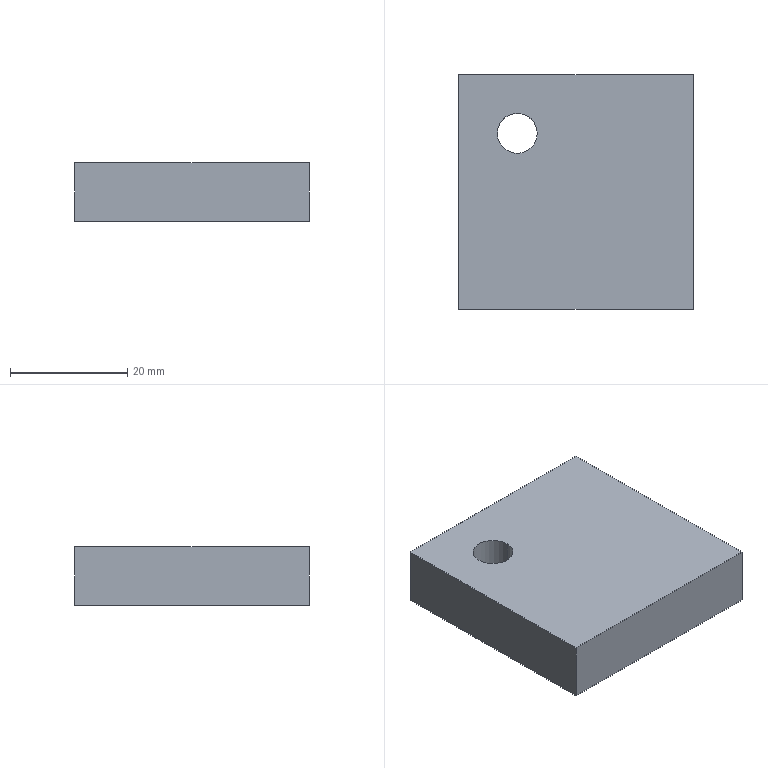Part | SolidWorks | features Extrusion 1, HoleWzd 1 | 1 solid | 8 faces | box 40 x 40 x 10 mm | volume 15637 mm3 | plane 6 | cylinder 2 | commonest cylinder face diameters 6.8 x2
STEP:
#1=CARTESIAN_POINT('',(-13.4,10.,-5.));
#2=VERTEX_POINT('',#1);
#3=CARTESIAN_POINT('',(-6.6,10.,-5.));
#4=VERTEX_POINT('',#3);
#5=CARTESIAN_POINT('',(-10.,10.,-5.));
#6=DIRECTION('',(0.,0.,1.));
#7=DIRECTION('',(1.,0.,0.));
#8=AXIS2_PLACEMENT_3D('',#5,#6,#7);
#9=CIRCLE('',#8,3.4);
#10=EDGE_CURVE('',#2,#4,#9,.T.);
#11=ORIENTED_EDGE('',*,*,#10,.F.);
#12=CARTESIAN_POINT('',(-13.4,10.,5.));
#13=VERTEX_POINT('',#12);
#14=CARTESIAN_POINT('',(-13.4,10.,5.));
#15=DIRECTION('',(0.,0.,1.));
#16=VECTOR('',#15,1000.);
#17=LINE('',#14,#16);
#18=EDGE_CURVE('',#2,#13,#17,.T.);
#19=ORIENTED_EDGE('',*,*,#18,.T.);
#20=CARTESIAN_POINT('',(-6.6,10.,5.));
#21=VERTEX_POINT('',#20);
#22=CARTESIAN_POINT('',(-10.,10.,5.));
#23=DIRECTION('',(0.,0.,1.));
#24=DIRECTION('',(1.,0.,0.));
#25=AXIS2_PLACEMENT_3D('',#22,#23,#24);
#26=CIRCLE('',#25,3.4);
#27=EDGE_CURVE('',#13,#21,#26,.T.);
#28=ORIENTED_EDGE('',*,*,#27,.T.);
#29=CARTESIAN_POINT('',(-6.6,10.,5.));
#30=DIRECTION('',(0.,0.,1.));
#31=VECTOR('',#30,1000.);
#32=LINE('',#29,#31);
#33=EDGE_CURVE('',#4,#21,#32,.T.);
#34=ORIENTED_EDGE('',*,*,#33,.F.);
#35=EDGE_LOOP('',(#11,#19,#28,#34));
#36=FACE_OUTER_BOUND('',#35,.T.);
#37=CARTESIAN_POINT('',(-10.,10.,5.));
#38=DIRECTION('',(0.,0.,1.));
#39=DIRECTION('',(1.,0.,0.));
#40=AXIS2_PLACEMENT_3D('',#37,#38,#39);
#41=CYLINDRICAL_SURFACE('',#40,3.4);
#42=ADVANCED_FACE('',(#36),#41,.F.);
#43=CARTESIAN_POINT('',(20.,-20.,-5.));
#44=VERTEX_POINT('',#43);
#45=CARTESIAN_POINT('',(20.,20.,-5.));
#46=VERTEX_POINT('',#45);
#47=CARTESIAN_POINT('',(20.,-20.,-5.));
#48=DIRECTION('',(0.,1.,0.));
#49=VECTOR('',#48,1000.);
#50=LINE('',#47,#49);
#51=EDGE_CURVE('',#44,#46,#50,.T.);
#52=ORIENTED_EDGE('',*,*,#51,.T.);
#53=CARTESIAN_POINT('',(20.,20.,5.));
#54=VERTEX_POINT('',#53);
#55=CARTESIAN_POINT('',(20.,20.,5.));
#56=DIRECTION('',(0.,0.,-1.));
#57=VECTOR('',#56,1000.);
#58=LINE('',#55,#57);
#59=EDGE_CURVE('',#54,#46,#58,.T.);
#60=ORIENTED_EDGE('',*,*,#59,.F.);
#61=CARTESIAN_POINT('',(20.,-20.,5.));
#62=VERTEX_POINT('',#61);
#63=CARTESIAN_POINT('',(20.,-20.,5.));
#64=DIRECTION('',(0.,1.,0.));
#65=VECTOR('',#64,1000.);
#66=LINE('',#63,#65);
#67=EDGE_CURVE('',#62,#54,#66,.T.);
#68=ORIENTED_EDGE('',*,*,#67,.F.);
#69=CARTESIAN_POINT('',(20.,-20.,5.));
#70=DIRECTION('',(0.,0.,-1.));
#71=VECTOR('',#70,1000.);
#72=LINE('',#69,#71);
#73=EDGE_CURVE('',#62,#44,#72,.T.);
#74=ORIENTED_EDGE('',*,*,#73,.T.);
#75=EDGE_LOOP('',(#52,#60,#68,#74));
#76=FACE_OUTER_BOUND('',#75,.T.);
#77=CARTESIAN_POINT('',(20.,-20.,5.));
#78=DIRECTION('',(-1.,0.,0.));
#79=DIRECTION('',(0.,0.,1.));
#80=AXIS2_PLACEMENT_3D('',#77,#78,#79);
#81=PLANE('',#80);
#82=ADVANCED_FACE('',(#76),#81,.F.);
#83=CARTESIAN_POINT('',(-20.,20.,-5.));
#84=VERTEX_POINT('',#83);
#85=CARTESIAN_POINT('',(-20.,20.,-5.));
#86=DIRECTION('',(-1.,0.,0.));
#87=VECTOR('',#86,1000.);
#88=LINE('',#85,#87);
#89=EDGE_CURVE('',#46,#84,#88,.T.);
#90=ORIENTED_EDGE('',*,*,#89,.T.);
#91=CARTESIAN_POINT('',(-20.,20.,5.));
#92=VERTEX_POINT('',#91);
#93=CARTESIAN_POINT('',(-20.,20.,5.));
#94=DIRECTION('',(0.,0.,-1.));
#95=VECTOR('',#94,1000.);
#96=LINE('',#93,#95);
#97=EDGE_CURVE('',#92,#84,#96,.T.);
#98=ORIENTED_EDGE('',*,*,#97,.F.);
#99=CARTESIAN_POINT('',(-20.,20.,5.));
#100=DIRECTION('',(-1.,0.,0.));
#101=VECTOR('',#100,1000.);
#102=LINE('',#99,#101);
#103=EDGE_CURVE('',#54,#92,#102,.T.);
#104=ORIENTED_EDGE('',*,*,#103,.F.);
#105=ORIENTED_EDGE('',*,*,#59,.T.);
#106=EDGE_LOOP('',(#90,#98,#104,#105));
#107=FACE_OUTER_BOUND('',#106,.T.);
#108=CARTESIAN_POINT('',(-20.,20.,5.));
#109=DIRECTION('',(0.,-1.,0.));
#110=DIRECTION('',(0.,0.,-1.));
#111=AXIS2_PLACEMENT_3D('',#108,#109,#110);
#112=PLANE('',#111);
#113=ADVANCED_FACE('',(#107),#112,.F.);
#114=CARTESIAN_POINT('',(-20.,-20.,-5.));
#115=VERTEX_POINT('',#114);
#116=CARTESIAN_POINT('',(-20.,-20.,-5.));
#117=DIRECTION('',(0.,-1.,0.));
#118=VECTOR('',#117,1000.);
#119=LINE('',#116,#118);
#120=EDGE_CURVE('',#84,#115,#119,.T.);
#121=ORIENTED_EDGE('',*,*,#120,.T.);
#122=CARTESIAN_POINT('',(-20.,-20.,5.));
#123=VERTEX_POINT('',#122);
#124=CARTESIAN_POINT('',(-20.,-20.,5.));
#125=DIRECTION('',(0.,0.,-1.));
#126=VECTOR('',#125,1000.);
#127=LINE('',#124,#126);
#128=EDGE_CURVE('',#123,#115,#127,.T.);
#129=ORIENTED_EDGE('',*,*,#128,.F.);
#130=CARTESIAN_POINT('',(-20.,-20.,5.));
#131=DIRECTION('',(0.,-1.,0.));
#132=VECTOR('',#131,1000.);
#133=LINE('',#130,#132);
#134=EDGE_CURVE('',#92,#123,#133,.T.);
#135=ORIENTED_EDGE('',*,*,#134,.F.);
#136=ORIENTED_EDGE('',*,*,#97,.T.);
#137=EDGE_LOOP('',(#121,#129,#135,#136));
#138=FACE_OUTER_BOUND('',#137,.T.);
#139=CARTESIAN_POINT('',(-20.,-20.,5.));
#140=DIRECTION('',(1.,0.,0.));
#141=DIRECTION('',(0.,0.,-1.));
#142=AXIS2_PLACEMENT_3D('',#139,#140,#141);
#143=PLANE('',#142);
#144=ADVANCED_FACE('',(#138),#143,.F.);
#145=CARTESIAN_POINT('',(-20.,-20.,-5.));
#146=DIRECTION('',(1.,0.,0.));
#147=VECTOR('',#146,1000.);
#148=LINE('',#145,#147);
#149=EDGE_CURVE('',#115,#44,#148,.T.);
#150=ORIENTED_EDGE('',*,*,#149,.T.);
#151=ORIENTED_EDGE('',*,*,#73,.F.);
#152=CARTESIAN_POINT('',(-20.,-20.,5.));
#153=DIRECTION('',(1.,0.,0.));
#154=VECTOR('',#153,1000.);
#155=LINE('',#152,#154);
#156=EDGE_CURVE('',#123,#62,#155,.T.);
#157=ORIENTED_EDGE('',*,*,#156,.F.);
#158=ORIENTED_EDGE('',*,*,#128,.T.);
#159=EDGE_LOOP('',(#150,#151,#157,#158));
#160=FACE_OUTER_BOUND('',#159,.T.);
#161=CARTESIAN_POINT('',(-20.,-20.,5.));
#162=DIRECTION('',(0.,1.,0.));
#163=DIRECTION('',(0.,0.,1.));
#164=AXIS2_PLACEMENT_3D('',#161,#162,#163);
#165=PLANE('',#164);
#166=ADVANCED_FACE('',(#160),#165,.F.);
#167=CARTESIAN_POINT('',(-10.,10.,5.));
#168=DIRECTION('',(0.,0.,1.));
#169=DIRECTION('',(1.,0.,0.));
#170=AXIS2_PLACEMENT_3D('',#167,#168,#169);
#171=CIRCLE('',#170,3.4);
#172=EDGE_CURVE('',#21,#13,#171,.T.);
#173=ORIENTED_EDGE('',*,*,#172,.F.);
#174=ORIENTED_EDGE('',*,*,#27,.F.);
#175=EDGE_LOOP('',(#173,#174));
#176=FACE_BOUND('',#175,.T.);
#177=ORIENTED_EDGE('',*,*,#67,.T.);
#178=ORIENTED_EDGE('',*,*,#103,.T.);
#179=ORIENTED_EDGE('',*,*,#134,.T.);
#180=ORIENTED_EDGE('',*,*,#156,.T.);
#181=EDGE_LOOP('',(#177,#178,#179,#180));
#182=FACE_OUTER_BOUND('',#181,.T.);
#183=CARTESIAN_POINT('',(0.,0.,5.));
#184=DIRECTION('',(0.,0.,-1.));
#185=DIRECTION('',(-1.,0.,0.));
#186=AXIS2_PLACEMENT_3D('',#183,#184,#185);
#187=PLANE('',#186);
#188=ADVANCED_FACE('',(#176,#182),#187,.F.);
#189=CARTESIAN_POINT('',(-10.,10.,-5.));
#190=DIRECTION('',(0.,0.,1.));
#191=DIRECTION('',(1.,0.,0.));
#192=AXIS2_PLACEMENT_3D('',#189,#190,#191);
#193=CIRCLE('',#192,3.4);
#194=EDGE_CURVE('',#4,#2,#193,.T.);
#195=ORIENTED_EDGE('',*,*,#194,.T.);
#196=ORIENTED_EDGE('',*,*,#10,.T.);
#197=EDGE_LOOP('',(#195,#196));
#198=FACE_BOUND('',#197,.T.);
#199=ORIENTED_EDGE('',*,*,#51,.F.);
#200=ORIENTED_EDGE('',*,*,#149,.F.);
#201=ORIENTED_EDGE('',*,*,#120,.F.);
#202=ORIENTED_EDGE('',*,*,#89,.F.);
#203=EDGE_LOOP('',(#199,#200,#201,#202));
#204=FACE_OUTER_BOUND('',#203,.T.);
#205=CARTESIAN_POINT('',(0.,0.,-5.));
#206=DIRECTION('',(0.,0.,-1.));
#207=DIRECTION('',(-1.,0.,0.));
#208=AXIS2_PLACEMENT_3D('',#205,#206,#207);
#209=PLANE('',#208);
#210=ADVANCED_FACE('',(#198,#204),#209,.T.);
#211=ORIENTED_EDGE('',*,*,#18,.F.);
#212=ORIENTED_EDGE('',*,*,#194,.F.);
#213=ORIENTED_EDGE('',*,*,#33,.T.);
#214=ORIENTED_EDGE('',*,*,#172,.T.);
#215=EDGE_LOOP('',(#211,#212,#213,#214));
#216=FACE_OUTER_BOUND('',#215,.T.);
#217=CARTESIAN_POINT('',(-10.,10.,5.));
#218=DIRECTION('',(0.,0.,1.));
#219=DIRECTION('',(1.,0.,0.));
#220=AXIS2_PLACEMENT_3D('',#217,#218,#219);
#221=CYLINDRICAL_SURFACE('',#220,3.4);
#222=ADVANCED_FACE('',(#216),#221,.F.);
#223=CLOSED_SHELL('',(#42,#82,#113,#144,#166,#188,#210,#222));
#224=MANIFOLD_SOLID_BREP('',#223);
#225=CARTESIAN_POINT('',(0.,0.,0.));
#226=DIRECTION('',(0.,0.,1.));
#227=DIRECTION('',(1.,0.,0.));
#228=AXIS2_PLACEMENT_3D('',#225,#226,#227);
#229=(LENGTH_UNIT()NAMED_UNIT(*)SI_UNIT(.MILLI.,.METRE.));
#230=UNCERTAINTY_MEASURE_WITH_UNIT(LENGTH_MEASURE(0.00001),#229,'','');
#231=(NAMED_UNIT(*)PLANE_ANGLE_UNIT()SI_UNIT($,.RADIAN.));
#232=(NAMED_UNIT(*)SI_UNIT($,.STERADIAN.)SOLID_ANGLE_UNIT());
#233=(GEOMETRIC_REPRESENTATION_CONTEXT(3)GLOBAL_UNCERTAINTY_ASSIGNED_CONTEXT((#230))GLOBAL_UNIT_ASSIGNED_CONTEXT((#229,#231,#232))REPRESENTATION_CONTEXT('',''));
#234=ADVANCED_BREP_SHAPE_REPRESENTATION('',(#224,#228),#233);